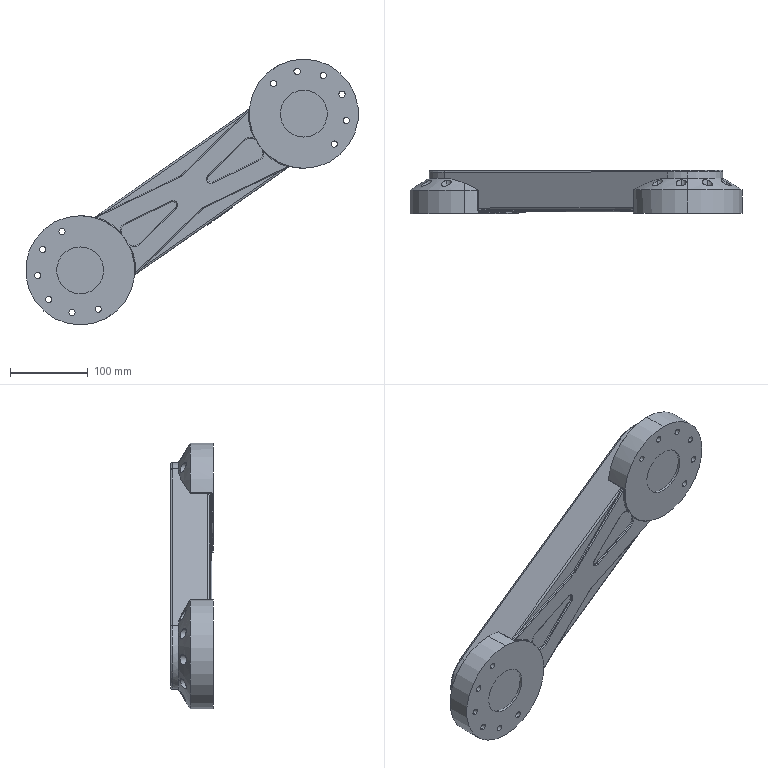Part | SolidWorks | features ICE 6, Fillet 5, Chamfer 1, CirPattern 1, Emboss 1, Extrusion 1, MirrorPattern 1 | 1 solid | 225 faces | box 426.703 x 55 x 340.752 mm | volume 1944571 mm3 | cylinder 89 | plane 64 | spline 49 | torus 17 | cone 6 | commonest cylinder face diameters 8 x24 13 x24 2.4 x13 20 x7 4 x4 60 x4